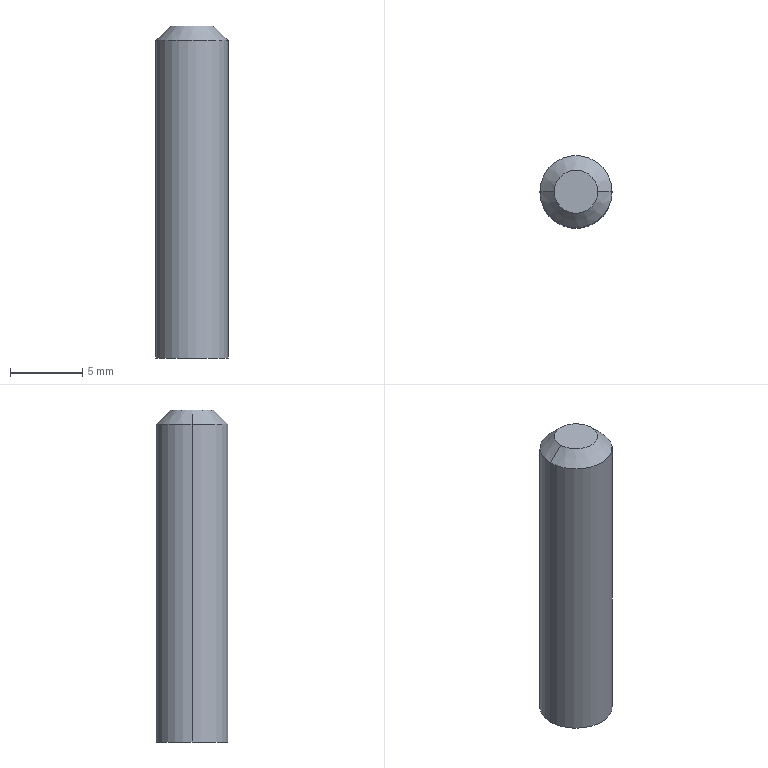Part | STEP file | rod_A_CJPB10_15_H4_0_ | 1 solid | 6 faces | box 5 x 5 x 23 mm | volume 444.797 mm3 | cylinder 2 | cone 2 | plane 2 | commonest cylinder face diameters 5 x2
STEP:
#1=CARTESIAN_POINT('',(2.5,0.,-11.));
#2=VERTEX_POINT('',#1);
#3=CARTESIAN_POINT('',(-2.5,0.,-11.));
#4=VERTEX_POINT('',#3);
#5=CARTESIAN_POINT('',(0.,0.,-11.));
#6=DIRECTION('',(0.,0.,1.));
#7=DIRECTION('',(1.,0.,0.));
#8=AXIS2_PLACEMENT_3D('',#5,#6,#7);
#9=CIRCLE('',#8,2.5);
#10=EDGE_CURVE('',#2,#4,#9,.T.);
#11=ORIENTED_EDGE('',*,*,#10,.T.);
#12=CARTESIAN_POINT('',(-2.5,0.,11.));
#13=VERTEX_POINT('',#12);
#14=CARTESIAN_POINT('',(-2.5,0.,-11.));
#15=DIRECTION('',(0.,0.,1.));
#16=VECTOR('',#15,1000.);
#17=LINE('',#14,#16);
#18=EDGE_CURVE('',#4,#13,#17,.T.);
#19=ORIENTED_EDGE('',*,*,#18,.T.);
#20=CARTESIAN_POINT('',(2.5,0.,11.));
#21=VERTEX_POINT('',#20);
#22=CARTESIAN_POINT('',(0.,0.,11.));
#23=DIRECTION('',(0.,0.,1.));
#24=DIRECTION('',(1.,0.,0.));
#25=AXIS2_PLACEMENT_3D('',#22,#23,#24);
#26=CIRCLE('',#25,2.5);
#27=EDGE_CURVE('',#21,#13,#26,.T.);
#28=ORIENTED_EDGE('',*,*,#27,.F.);
#29=CARTESIAN_POINT('',(2.5,0.,-11.));
#30=DIRECTION('',(0.,0.,1.));
#31=VECTOR('',#30,1000.);
#32=LINE('',#29,#31);
#33=EDGE_CURVE('',#2,#21,#32,.T.);
#34=ORIENTED_EDGE('',*,*,#33,.F.);
#35=EDGE_LOOP('',(#11,#19,#28,#34));
#36=FACE_OUTER_BOUND('',#35,.T.);
#37=CARTESIAN_POINT('',(0.,0.,-11.));
#38=DIRECTION('',(0.,0.,1.));
#39=DIRECTION('',(1.,0.,0.));
#40=AXIS2_PLACEMENT_3D('',#37,#38,#39);
#41=CYLINDRICAL_SURFACE('',#40,2.5);
#42=ADVANCED_FACE('',(#36),#41,.T.);
#43=CARTESIAN_POINT('',(1.5,0.,12.));
#44=VERTEX_POINT('',#43);
#45=CARTESIAN_POINT('',(-1.5,0.,12.));
#46=VERTEX_POINT('',#45);
#47=CARTESIAN_POINT('',(0.,0.,12.));
#48=DIRECTION('',(0.,0.,1.));
#49=DIRECTION('',(1.,0.,0.));
#50=AXIS2_PLACEMENT_3D('',#47,#48,#49);
#51=CIRCLE('',#50,1.5);
#52=EDGE_CURVE('',#44,#46,#51,.T.);
#53=ORIENTED_EDGE('',*,*,#52,.F.);
#54=CARTESIAN_POINT('',(2.5,0.,11.));
#55=DIRECTION('',(0.7071,0.,-0.7071));
#56=VECTOR('',#55,1000.);
#57=LINE('',#54,#56);
#58=EDGE_CURVE('',#44,#21,#57,.T.);
#59=ORIENTED_EDGE('',*,*,#58,.T.);
#60=ORIENTED_EDGE('',*,*,#27,.T.);
#61=CARTESIAN_POINT('',(-2.5,0.,11.));
#62=DIRECTION('',(-0.7071,0.,-0.7071));
#63=VECTOR('',#62,1000.);
#64=LINE('',#61,#63);
#65=EDGE_CURVE('',#46,#13,#64,.T.);
#66=ORIENTED_EDGE('',*,*,#65,.F.);
#67=EDGE_LOOP('',(#53,#59,#60,#66));
#68=FACE_OUTER_BOUND('',#67,.T.);
#69=CARTESIAN_POINT('',(0.,0.,11.));
#70=DIRECTION('',(0.,0.,-1.));
#71=DIRECTION('',(-1.,0.,0.));
#72=AXIS2_PLACEMENT_3D('',#69,#70,#71);
#73=CONICAL_SURFACE('',#72,2.5,0.7854);
#74=ADVANCED_FACE('',(#68),#73,.T.);
#75=CARTESIAN_POINT('',(0.,0.,12.));
#76=DIRECTION('',(0.,0.,1.));
#77=DIRECTION('',(1.,0.,0.));
#78=AXIS2_PLACEMENT_3D('',#75,#76,#77);
#79=CIRCLE('',#78,1.5);
#80=EDGE_CURVE('',#46,#44,#79,.T.);
#81=ORIENTED_EDGE('',*,*,#80,.T.);
#82=ORIENTED_EDGE('',*,*,#52,.T.);
#83=EDGE_LOOP('',(#81,#82));
#84=FACE_OUTER_BOUND('',#83,.T.);
#85=CARTESIAN_POINT('',(0.,0.,12.));
#86=DIRECTION('',(0.,0.,-1.));
#87=DIRECTION('',(-1.,0.,0.));
#88=AXIS2_PLACEMENT_3D('',#85,#86,#87);
#89=PLANE('',#88);
#90=ADVANCED_FACE('',(#84),#89,.F.);
#91=ORIENTED_EDGE('',*,*,#58,.F.);
#92=ORIENTED_EDGE('',*,*,#80,.F.);
#93=ORIENTED_EDGE('',*,*,#65,.T.);
#94=CARTESIAN_POINT('',(0.,0.,11.));
#95=DIRECTION('',(0.,0.,1.));
#96=DIRECTION('',(1.,0.,0.));
#97=AXIS2_PLACEMENT_3D('',#94,#95,#96);
#98=CIRCLE('',#97,2.5);
#99=EDGE_CURVE('',#13,#21,#98,.T.);
#100=ORIENTED_EDGE('',*,*,#99,.T.);
#101=EDGE_LOOP('',(#91,#92,#93,#100));
#102=FACE_OUTER_BOUND('',#101,.T.);
#103=CARTESIAN_POINT('',(0.,0.,11.));
#104=DIRECTION('',(0.,0.,-1.));
#105=DIRECTION('',(-1.,0.,0.));
#106=AXIS2_PLACEMENT_3D('',#103,#104,#105);
#107=CONICAL_SURFACE('',#106,2.5,0.7854);
#108=ADVANCED_FACE('',(#102),#107,.T.);
#109=ORIENTED_EDGE('',*,*,#18,.F.);
#110=CARTESIAN_POINT('',(0.,0.,-11.));
#111=DIRECTION('',(0.,0.,1.));
#112=DIRECTION('',(1.,0.,0.));
#113=AXIS2_PLACEMENT_3D('',#110,#111,#112);
#114=CIRCLE('',#113,2.5);
#115=EDGE_CURVE('',#4,#2,#114,.T.);
#116=ORIENTED_EDGE('',*,*,#115,.T.);
#117=ORIENTED_EDGE('',*,*,#33,.T.);
#118=ORIENTED_EDGE('',*,*,#99,.F.);
#119=EDGE_LOOP('',(#109,#116,#117,#118));
#120=FACE_OUTER_BOUND('',#119,.T.);
#121=CARTESIAN_POINT('',(0.,0.,-11.));
#122=DIRECTION('',(0.,0.,1.));
#123=DIRECTION('',(1.,0.,0.));
#124=AXIS2_PLACEMENT_3D('',#121,#122,#123);
#125=CYLINDRICAL_SURFACE('',#124,2.5);
#126=ADVANCED_FACE('',(#120),#125,.T.);
#127=ORIENTED_EDGE('',*,*,#10,.F.);
#128=ORIENTED_EDGE('',*,*,#115,.F.);
#129=EDGE_LOOP('',(#127,#128));
#130=FACE_OUTER_BOUND('',#129,.T.);
#131=CARTESIAN_POINT('',(0.,2.5,-11.));
#132=DIRECTION('',(0.,0.,1.));
#133=DIRECTION('',(1.,0.,0.));
#134=AXIS2_PLACEMENT_3D('',#131,#132,#133);
#135=PLANE('',#134);
#136=ADVANCED_FACE('',(#130),#135,.F.);
#137=CLOSED_SHELL('',(#42,#74,#90,#108,#126,#136));
#138=MANIFOLD_SOLID_BREP('',#137);
#139=CARTESIAN_POINT('',(0.,0.,0.));
#140=DIRECTION('',(0.,0.,1.));
#141=DIRECTION('',(1.,0.,0.));
#142=AXIS2_PLACEMENT_3D('',#139,#140,#141);
#143=(LENGTH_UNIT()NAMED_UNIT(*)SI_UNIT(.MILLI.,.METRE.));
#144=UNCERTAINTY_MEASURE_WITH_UNIT(LENGTH_MEASURE(0.00001),#143,'','');
#145=(NAMED_UNIT(*)PLANE_ANGLE_UNIT()SI_UNIT($,.RADIAN.));
#146=(NAMED_UNIT(*)SI_UNIT($,.STERADIAN.)SOLID_ANGLE_UNIT());
#147=(GEOMETRIC_REPRESENTATION_CONTEXT(3)GLOBAL_UNCERTAINTY_ASSIGNED_CONTEXT((#144))GLOBAL_UNIT_ASSIGNED_CONTEXT((#143,#145,#146))REPRESENTATION_CONTEXT('',''));
#148=ADVANCED_BREP_SHAPE_REPRESENTATION('',(#138,#142),#147);